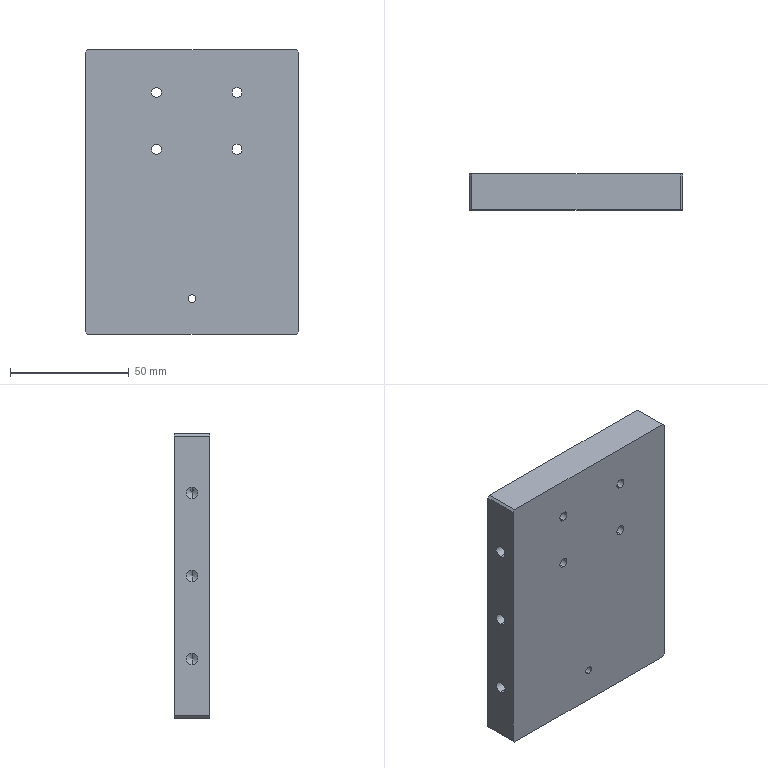Part | SolidWorks | features BaseBody 1 | 1 solid | 40 faces | box 90 x 15 x 120 mm | volume 159292 mm3 | cylinder 20 | cone 10 | plane 10 | commonest cylinder face diameters 5 x10 4.2 x8 3.3 x2
STEP:
#1=CARTESIAN_POINT('',(64.,15.,-39.9));
#2=VERTEX_POINT('',#1);
#3=CARTESIAN_POINT('',(64.,15.,-44.1));
#4=VERTEX_POINT('',#3);
#5=CARTESIAN_POINT('',(64.,15.,-42.));
#6=DIRECTION('',(0.,-1.,0.));
#7=DIRECTION('',(0.,0.,-1.));
#8=AXIS2_PLACEMENT_3D('',#5,#6,#7);
#9=CIRCLE('',#8,2.1);
#10=EDGE_CURVE('',#2,#4,#9,.T.);
#11=ORIENTED_EDGE('',*,*,#10,.F.);
#12=CARTESIAN_POINT('',(64.,0.,-39.9));
#13=VERTEX_POINT('',#12);
#14=CARTESIAN_POINT('',(64.,0.,-39.9));
#15=DIRECTION('',(0.,-1.,0.));
#16=VECTOR('',#15,1000.);
#17=LINE('',#14,#16);
#18=EDGE_CURVE('',#2,#13,#17,.T.);
#19=ORIENTED_EDGE('',*,*,#18,.T.);
#20=CARTESIAN_POINT('',(64.,0.,-44.1));
#21=VERTEX_POINT('',#20);
#22=CARTESIAN_POINT('',(64.,0.,-42.));
#23=DIRECTION('',(0.,1.,0.));
#24=DIRECTION('',(0.,0.,-1.));
#25=AXIS2_PLACEMENT_3D('',#22,#23,#24);
#26=CIRCLE('',#25,2.1);
#27=EDGE_CURVE('',#21,#13,#26,.T.);
#28=ORIENTED_EDGE('',*,*,#27,.F.);
#29=CARTESIAN_POINT('',(64.,0.,-44.1));
#30=DIRECTION('',(0.,-1.,0.));
#31=VECTOR('',#30,1000.);
#32=LINE('',#29,#31);
#33=EDGE_CURVE('',#4,#21,#32,.T.);
#34=ORIENTED_EDGE('',*,*,#33,.F.);
#35=EDGE_LOOP('',(#11,#19,#28,#34));
#36=FACE_OUTER_BOUND('',#35,.T.);
#37=CARTESIAN_POINT('',(64.,0.,-42.));
#38=DIRECTION('',(0.,-1.,0.));
#39=DIRECTION('',(0.,0.,-1.));
#40=AXIS2_PLACEMENT_3D('',#37,#38,#39);
#41=CYLINDRICAL_SURFACE('',#40,2.1);
#42=ADVANCED_FACE('',(#36),#41,.F.);
#43=CARTESIAN_POINT('',(64.,15.,-15.9));
#44=VERTEX_POINT('',#43);
#45=CARTESIAN_POINT('',(64.,15.,-20.1));
#46=VERTEX_POINT('',#45);
#47=CARTESIAN_POINT('',(64.,15.,-18.));
#48=DIRECTION('',(0.,-1.,0.));
#49=DIRECTION('',(0.,0.,-1.));
#50=AXIS2_PLACEMENT_3D('',#47,#48,#49);
#51=CIRCLE('',#50,2.1);
#52=EDGE_CURVE('',#44,#46,#51,.T.);
#53=ORIENTED_EDGE('',*,*,#52,.F.);
#54=CARTESIAN_POINT('',(64.,0.,-15.9));
#55=VERTEX_POINT('',#54);
#56=CARTESIAN_POINT('',(64.,0.,-15.9));
#57=DIRECTION('',(0.,-1.,0.));
#58=VECTOR('',#57,1000.);
#59=LINE('',#56,#58);
#60=EDGE_CURVE('',#44,#55,#59,.T.);
#61=ORIENTED_EDGE('',*,*,#60,.T.);
#62=CARTESIAN_POINT('',(64.,0.,-20.1));
#63=VERTEX_POINT('',#62);
#64=CARTESIAN_POINT('',(64.,0.,-18.));
#65=DIRECTION('',(0.,1.,0.));
#66=DIRECTION('',(0.,0.,-1.));
#67=AXIS2_PLACEMENT_3D('',#64,#65,#66);
#68=CIRCLE('',#67,2.1);
#69=EDGE_CURVE('',#63,#55,#68,.T.);
#70=ORIENTED_EDGE('',*,*,#69,.F.);
#71=CARTESIAN_POINT('',(64.,0.,-20.1));
#72=DIRECTION('',(0.,-1.,0.));
#73=VECTOR('',#72,1000.);
#74=LINE('',#71,#73);
#75=EDGE_CURVE('',#46,#63,#74,.T.);
#76=ORIENTED_EDGE('',*,*,#75,.F.);
#77=EDGE_LOOP('',(#53,#61,#70,#76));
#78=FACE_OUTER_BOUND('',#77,.T.);
#79=CARTESIAN_POINT('',(64.,0.,-18.));
#80=DIRECTION('',(0.,-1.,0.));
#81=DIRECTION('',(0.,0.,-1.));
#82=AXIS2_PLACEMENT_3D('',#79,#80,#81);
#83=CYLINDRICAL_SURFACE('',#82,2.1);
#84=ADVANCED_FACE('',(#78),#83,.F.);
#85=CARTESIAN_POINT('',(30.,15.,-15.9));
#86=VERTEX_POINT('',#85);
#87=CARTESIAN_POINT('',(30.,15.,-20.1));
#88=VERTEX_POINT('',#87);
#89=CARTESIAN_POINT('',(30.,15.,-18.));
#90=DIRECTION('',(0.,-1.,0.));
#91=DIRECTION('',(0.,0.,-1.));
#92=AXIS2_PLACEMENT_3D('',#89,#90,#91);
#93=CIRCLE('',#92,2.1);
#94=EDGE_CURVE('',#86,#88,#93,.T.);
#95=ORIENTED_EDGE('',*,*,#94,.F.);
#96=CARTESIAN_POINT('',(30.,0.,-15.9));
#97=VERTEX_POINT('',#96);
#98=CARTESIAN_POINT('',(30.,0.,-15.9));
#99=DIRECTION('',(0.,-1.,0.));
#100=VECTOR('',#99,1000.);
#101=LINE('',#98,#100);
#102=EDGE_CURVE('',#86,#97,#101,.T.);
#103=ORIENTED_EDGE('',*,*,#102,.T.);
#104=CARTESIAN_POINT('',(30.,0.,-20.1));
#105=VERTEX_POINT('',#104);
#106=CARTESIAN_POINT('',(30.,0.,-18.));
#107=DIRECTION('',(0.,1.,0.));
#108=DIRECTION('',(0.,0.,-1.));
#109=AXIS2_PLACEMENT_3D('',#106,#107,#108);
#110=CIRCLE('',#109,2.1);
#111=EDGE_CURVE('',#105,#97,#110,.T.);
#112=ORIENTED_EDGE('',*,*,#111,.F.);
#113=CARTESIAN_POINT('',(30.,0.,-20.1));
#114=DIRECTION('',(0.,-1.,0.));
#115=VECTOR('',#114,1000.);
#116=LINE('',#113,#115);
#117=EDGE_CURVE('',#88,#105,#116,.T.);
#118=ORIENTED_EDGE('',*,*,#117,.F.);
#119=EDGE_LOOP('',(#95,#103,#112,#118));
#120=FACE_OUTER_BOUND('',#119,.T.);
#121=CARTESIAN_POINT('',(30.,0.,-18.));
#122=DIRECTION('',(0.,-1.,0.));
#123=DIRECTION('',(0.,0.,-1.));
#124=AXIS2_PLACEMENT_3D('',#121,#122,#123);
#125=CYLINDRICAL_SURFACE('',#124,2.1);
#126=ADVANCED_FACE('',(#120),#125,.F.);
#127=CARTESIAN_POINT('',(30.,15.,-39.9));
#128=VERTEX_POINT('',#127);
#129=CARTESIAN_POINT('',(30.,15.,-44.1));
#130=VERTEX_POINT('',#129);
#131=CARTESIAN_POINT('',(30.,15.,-42.));
#132=DIRECTION('',(0.,-1.,0.));
#133=DIRECTION('',(0.,0.,-1.));
#134=AXIS2_PLACEMENT_3D('',#131,#132,#133);
#135=CIRCLE('',#134,2.1);
#136=EDGE_CURVE('',#128,#130,#135,.T.);
#137=ORIENTED_EDGE('',*,*,#136,.F.);
#138=CARTESIAN_POINT('',(30.,0.,-39.9));
#139=VERTEX_POINT('',#138);
#140=CARTESIAN_POINT('',(30.,0.,-39.9));
#141=DIRECTION('',(0.,-1.,0.));
#142=VECTOR('',#141,1000.);
#143=LINE('',#140,#142);
#144=EDGE_CURVE('',#128,#139,#143,.T.);
#145=ORIENTED_EDGE('',*,*,#144,.T.);
#146=CARTESIAN_POINT('',(30.,0.,-44.1));
#147=VERTEX_POINT('',#146);
#148=CARTESIAN_POINT('',(30.,0.,-42.));
#149=DIRECTION('',(0.,1.,0.));
#150=DIRECTION('',(0.,0.,-1.));
#151=AXIS2_PLACEMENT_3D('',#148,#149,#150);
#152=CIRCLE('',#151,2.1);
#153=EDGE_CURVE('',#147,#139,#152,.T.);
#154=ORIENTED_EDGE('',*,*,#153,.F.);
#155=CARTESIAN_POINT('',(30.,0.,-44.1));
#156=DIRECTION('',(0.,-1.,0.));
#157=VECTOR('',#156,1000.);
#158=LINE('',#155,#157);
#159=EDGE_CURVE('',#130,#147,#158,.T.);
#160=ORIENTED_EDGE('',*,*,#159,.F.);
#161=EDGE_LOOP('',(#137,#145,#154,#160));
#162=FACE_OUTER_BOUND('',#161,.T.);
#163=CARTESIAN_POINT('',(30.,0.,-42.));
#164=DIRECTION('',(0.,-1.,0.));
#165=DIRECTION('',(0.,0.,-1.));
#166=AXIS2_PLACEMENT_3D('',#163,#164,#165);
#167=CYLINDRICAL_SURFACE('',#166,2.1);
#168=ADVANCED_FACE('',(#162),#167,.F.);
#169=CARTESIAN_POINT('',(45.,0.,-106.65));
#170=VERTEX_POINT('',#169);
#171=CARTESIAN_POINT('',(45.,0.,-103.35));
#172=VERTEX_POINT('',#171);
#173=CARTESIAN_POINT('',(45.,0.,-105.));
#174=DIRECTION('',(0.,1.,0.));
#175=DIRECTION('',(0.,0.,1.));
#176=AXIS2_PLACEMENT_3D('',#173,#174,#175);
#177=CIRCLE('',#176,1.65);
#178=EDGE_CURVE('',#170,#172,#177,.T.);
#179=ORIENTED_EDGE('',*,*,#178,.F.);
#180=CARTESIAN_POINT('',(45.,15.,-106.65));
#181=VERTEX_POINT('',#180);
#182=CARTESIAN_POINT('',(45.,15.,-106.65));
#183=DIRECTION('',(0.,1.,0.));
#184=VECTOR('',#183,1000.);
#185=LINE('',#182,#184);
#186=EDGE_CURVE('',#170,#181,#185,.T.);
#187=ORIENTED_EDGE('',*,*,#186,.T.);
#188=CARTESIAN_POINT('',(45.,15.,-103.35));
#189=VERTEX_POINT('',#188);
#190=CARTESIAN_POINT('',(45.,15.,-105.));
#191=DIRECTION('',(0.,-1.,0.));
#192=DIRECTION('',(0.,0.,1.));
#193=AXIS2_PLACEMENT_3D('',#190,#191,#192);
#194=CIRCLE('',#193,1.65);
#195=EDGE_CURVE('',#189,#181,#194,.T.);
#196=ORIENTED_EDGE('',*,*,#195,.F.);
#197=CARTESIAN_POINT('',(45.,15.,-103.35));
#198=DIRECTION('',(0.,1.,0.));
#199=VECTOR('',#198,1000.);
#200=LINE('',#197,#199);
#201=EDGE_CURVE('',#172,#189,#200,.T.);
#202=ORIENTED_EDGE('',*,*,#201,.F.);
#203=EDGE_LOOP('',(#179,#187,#196,#202));
#204=FACE_OUTER_BOUND('',#203,.T.);
#205=CARTESIAN_POINT('',(45.,15.,-105.));
#206=DIRECTION('',(0.,1.,0.));
#207=DIRECTION('',(0.,0.,1.));
#208=AXIS2_PLACEMENT_3D('',#205,#206,#207);
#209=CYLINDRICAL_SURFACE('',#208,1.65);
#210=ADVANCED_FACE('',(#204),#209,.F.);
#211=CARTESIAN_POINT('',(77.5,7.5,-103.));
#212=VERTEX_POINT('',#211);
#213=CARTESIAN_POINT('',(75.,5.,-103.));
#214=VERTEX_POINT('',#213);
#215=CARTESIAN_POINT('',(75.,7.5,-103.));
#216=DIRECTION('',(0.,0.,-1.));
#217=DIRECTION('',(-1.,0.,0.));
#218=AXIS2_PLACEMENT_3D('',#215,#216,#217);
#219=CIRCLE('',#218,2.5);
#220=EDGE_CURVE('',#212,#214,#219,.T.);
#221=ORIENTED_EDGE('',*,*,#220,.F.);
#222=CARTESIAN_POINT('',(77.5,7.5,-120.));
#223=VERTEX_POINT('',#222);
#224=CARTESIAN_POINT('',(77.5,7.5,-120.));
#225=DIRECTION('',(0.,0.,-1.));
#226=VECTOR('',#225,1000.);
#227=LINE('',#224,#226);
#228=EDGE_CURVE('',#212,#223,#227,.T.);
#229=ORIENTED_EDGE('',*,*,#228,.T.);
#230=CARTESIAN_POINT('',(72.5,7.5,-120.));
#231=VERTEX_POINT('',#230);
#232=CARTESIAN_POINT('',(75.,7.5,-120.));
#233=DIRECTION('',(0.,0.,-1.));
#234=DIRECTION('',(-1.,0.,0.));
#235=AXIS2_PLACEMENT_3D('',#232,#233,#234);
#236=CIRCLE('',#235,2.5);
#237=EDGE_CURVE('',#223,#231,#236,.T.);
#238=ORIENTED_EDGE('',*,*,#237,.T.);
#239=CARTESIAN_POINT('',(72.5,7.5,-103.));
#240=VERTEX_POINT('',#239);
#241=CARTESIAN_POINT('',(72.5,7.5,-120.));
#242=DIRECTION('',(0.,0.,-1.));
#243=VECTOR('',#242,1000.);
#244=LINE('',#241,#243);
#245=EDGE_CURVE('',#240,#231,#244,.T.);
#246=ORIENTED_EDGE('',*,*,#245,.F.);
#247=CARTESIAN_POINT('',(75.,7.5,-103.));
#248=DIRECTION('',(0.,0.,-1.));
#249=DIRECTION('',(-1.,0.,0.));
#250=AXIS2_PLACEMENT_3D('',#247,#248,#249);
#251=CIRCLE('',#250,2.5);
#252=EDGE_CURVE('',#214,#240,#251,.T.);
#253=ORIENTED_EDGE('',*,*,#252,.F.);
#254=EDGE_LOOP('',(#221,#229,#238,#246,#253));
#255=FACE_OUTER_BOUND('',#254,.T.);
#256=CARTESIAN_POINT('',(75.,7.5,-120.));
#257=DIRECTION('',(0.,0.,-1.));
#258=DIRECTION('',(-1.,0.,0.));
#259=AXIS2_PLACEMENT_3D('',#256,#257,#258);
#260=CYLINDRICAL_SURFACE('',#259,2.5);
#261=ADVANCED_FACE('',(#255),#260,.F.);
#262=CARTESIAN_POINT('',(17.5,7.5,-103.));
#263=VERTEX_POINT('',#262);
#264=CARTESIAN_POINT('',(12.5,7.5,-103.));
#265=VERTEX_POINT('',#264);
#266=CARTESIAN_POINT('',(15.,7.5,-103.));
#267=DIRECTION('',(0.,0.,-1.));
#268=DIRECTION('',(-1.,0.,0.));
#269=AXIS2_PLACEMENT_3D('',#266,#267,#268);
#270=CIRCLE('',#269,2.5);
#271=EDGE_CURVE('',#263,#265,#270,.T.);
#272=ORIENTED_EDGE('',*,*,#271,.F.);
#273=CARTESIAN_POINT('',(17.5,7.5,-120.));
#274=VERTEX_POINT('',#273);
#275=CARTESIAN_POINT('',(17.5,7.5,-120.));
#276=DIRECTION('',(0.,0.,-1.));
#277=VECTOR('',#276,1000.);
#278=LINE('',#275,#277);
#279=EDGE_CURVE('',#263,#274,#278,.T.);
#280=ORIENTED_EDGE('',*,*,#279,.T.);
#281=CARTESIAN_POINT('',(12.5,7.5,-120.));
#282=VERTEX_POINT('',#281);
#283=CARTESIAN_POINT('',(15.,7.5,-120.));
#284=DIRECTION('',(0.,0.,-1.));
#285=DIRECTION('',(-1.,0.,0.));
#286=AXIS2_PLACEMENT_3D('',#283,#284,#285);
#287=CIRCLE('',#286,2.5);
#288=EDGE_CURVE('',#274,#282,#287,.T.);
#289=ORIENTED_EDGE('',*,*,#288,.T.);
#290=CARTESIAN_POINT('',(12.5,7.5,-120.));
#291=DIRECTION('',(0.,0.,-1.));
#292=VECTOR('',#291,1000.);
#293=LINE('',#290,#292);
#294=EDGE_CURVE('',#265,#282,#293,.T.);
#295=ORIENTED_EDGE('',*,*,#294,.F.);
#296=EDGE_LOOP('',(#272,#280,#289,#295));
#297=FACE_OUTER_BOUND('',#296,.T.);
#298=CARTESIAN_POINT('',(15.,7.5,-120.));
#299=DIRECTION('',(0.,0.,-1.));
#300=DIRECTION('',(-1.,0.,0.));
#301=AXIS2_PLACEMENT_3D('',#298,#299,#300);
#302=CYLINDRICAL_SURFACE('',#301,2.5);
#303=ADVANCED_FACE('',(#297),#302,.F.);
#304=CARTESIAN_POINT('',(17.,7.5,-27.5));
#305=VERTEX_POINT('',#304);
#306=CARTESIAN_POINT('',(17.,7.5,-22.5));
#307=VERTEX_POINT('',#306);
#308=CARTESIAN_POINT('',(17.,7.5,-25.));
#309=DIRECTION('',(-1.,0.,0.));
#310=DIRECTION('',(0.,0.,1.));
#311=AXIS2_PLACEMENT_3D('',#308,#309,#310);
#312=CIRCLE('',#311,2.5);
#313=EDGE_CURVE('',#305,#307,#312,.T.);
#314=ORIENTED_EDGE('',*,*,#313,.F.);
#315=CARTESIAN_POINT('',(0.,7.5,-27.5));
#316=VERTEX_POINT('',#315);
#317=CARTESIAN_POINT('',(0.,7.5,-27.5));
#318=DIRECTION('',(-1.,0.,0.));
#319=VECTOR('',#318,1000.);
#320=LINE('',#317,#319);
#321=EDGE_CURVE('',#305,#316,#320,.T.);
#322=ORIENTED_EDGE('',*,*,#321,.T.);
#323=CARTESIAN_POINT('',(0.,7.5,-22.5));
#324=VERTEX_POINT('',#323);
#325=CARTESIAN_POINT('',(0.,7.5,-25.));
#326=DIRECTION('',(-1.,0.,0.));
#327=DIRECTION('',(0.,0.,1.));
#328=AXIS2_PLACEMENT_3D('',#325,#326,#327);
#329=CIRCLE('',#328,2.5);
#330=EDGE_CURVE('',#316,#324,#329,.T.);
#331=ORIENTED_EDGE('',*,*,#330,.T.);
#332=CARTESIAN_POINT('',(0.,7.5,-22.5));
#333=DIRECTION('',(-1.,0.,0.));
#334=VECTOR('',#333,1000.);
#335=LINE('',#332,#334);
#336=EDGE_CURVE('',#307,#324,#335,.T.);
#337=ORIENTED_EDGE('',*,*,#336,.F.);
#338=EDGE_LOOP('',(#314,#322,#331,#337));
#339=FACE_OUTER_BOUND('',#338,.T.);
#340=CARTESIAN_POINT('',(0.,7.5,-25.));
#341=DIRECTION('',(-1.,0.,0.));
#342=DIRECTION('',(0.,0.,1.));
#343=AXIS2_PLACEMENT_3D('',#340,#341,#342);
#344=CYLINDRICAL_SURFACE('',#343,2.5);
#345=ADVANCED_FACE('',(#339),#344,.F.);
#346=CARTESIAN_POINT('',(17.,7.5,-97.5));
#347=VERTEX_POINT('',#346);
#348=CARTESIAN_POINT('',(17.,7.5,-92.5));
#349=VERTEX_POINT('',#348);
#350=CARTESIAN_POINT('',(17.,7.5,-95.));
#351=DIRECTION('',(-1.,0.,0.));
#352=DIRECTION('',(0.,0.,1.));
#353=AXIS2_PLACEMENT_3D('',#350,#351,#352);
#354=CIRCLE('',#353,2.5);
#355=EDGE_CURVE('',#347,#349,#354,.T.);
#356=ORIENTED_EDGE('',*,*,#355,.F.);
#357=CARTESIAN_POINT('',(0.,7.5,-97.5));
#358=VERTEX_POINT('',#357);
#359=CARTESIAN_POINT('',(0.,7.5,-97.5));
#360=DIRECTION('',(-1.,0.,0.));
#361=VECTOR('',#360,1000.);
#362=LINE('',#359,#361);
#363=EDGE_CURVE('',#347,#358,#362,.T.);
#364=ORIENTED_EDGE('',*,*,#363,.T.);
#365=CARTESIAN_POINT('',(0.,7.5,-92.5));
#366=VERTEX_POINT('',#365);
#367=CARTESIAN_POINT('',(0.,7.5,-95.));
#368=DIRECTION('',(-1.,0.,0.));
#369=DIRECTION('',(0.,0.,1.));
#370=AXIS2_PLACEMENT_3D('',#367,#368,#369);
#371=CIRCLE('',#370,2.5);
#372=EDGE_CURVE('',#358,#366,#371,.T.);
#373=ORIENTED_EDGE('',*,*,#372,.T.);
#374=CARTESIAN_POINT('',(0.,7.5,-92.5));
#375=DIRECTION('',(-1.,0.,0.));
#376=VECTOR('',#375,1000.);
#377=LINE('',#374,#376);
#378=EDGE_CURVE('',#349,#366,#377,.T.);
#379=ORIENTED_EDGE('',*,*,#378,.F.);
#380=EDGE_LOOP('',(#356,#364,#373,#379));
#381=FACE_OUTER_BOUND('',#380,.T.);
#382=CARTESIAN_POINT('',(0.,7.5,-95.));
#383=DIRECTION('',(-1.,0.,0.));
#384=DIRECTION('',(0.,0.,1.));
#385=AXIS2_PLACEMENT_3D('',#382,#383,#384);
#386=CYLINDRICAL_SURFACE('',#385,2.5);
#387=ADVANCED_FACE('',(#381),#386,.F.);
#388=CARTESIAN_POINT('',(17.,7.5,-62.5));
#389=VERTEX_POINT('',#388);
#390=CARTESIAN_POINT('',(17.,7.5,-57.5));
#391=VERTEX_POINT('',#390);
#392=CARTESIAN_POINT('',(17.,7.5,-60.));
#393=DIRECTION('',(-1.,0.,0.));
#394=DIRECTION('',(0.,0.,1.));
#395=AXIS2_PLACEMENT_3D('',#392,#393,#394);
#396=CIRCLE('',#395,2.5);
#397=EDGE_CURVE('',#389,#391,#396,.T.);
#398=ORIENTED_EDGE('',*,*,#397,.F.);
#399=CARTESIAN_POINT('',(0.,7.5,-62.5));
#400=VERTEX_POINT('',#399);
#401=CARTESIAN_POINT('',(0.,7.5,-62.5));
#402=DIRECTION('',(-1.,0.,0.));
#403=VECTOR('',#402,1000.);
#404=LINE('',#401,#403);
#405=EDGE_CURVE('',#389,#400,#404,.T.);
#406=ORIENTED_EDGE('',*,*,#405,.T.);
#407=CARTESIAN_POINT('',(0.,7.5,-57.5));
#408=VERTEX_POINT('',#407);
#409=CARTESIAN_POINT('',(0.,7.5,-60.));
#410=DIRECTION('',(-1.,0.,0.));
#411=DIRECTION('',(0.,0.,1.));
#412=AXIS2_PLACEMENT_3D('',#409,#410,#411);
#413=CIRCLE('',#412,2.5);
#414=EDGE_CURVE('',#400,#408,#413,.T.);
#415=ORIENTED_EDGE('',*,*,#414,.T.);
#416=CARTESIAN_POINT('',(0.,7.5,-57.5));
#417=DIRECTION('',(-1.,0.,0.));
#418=VECTOR('',#417,1000.);
#419=LINE('',#416,#418);
#420=EDGE_CURVE('',#391,#408,#419,.T.);
#421=ORIENTED_EDGE('',*,*,#420,.F.);
#422=EDGE_LOOP('',(#398,#406,#415,#421));
#423=FACE_OUTER_BOUND('',#422,.T.);
#424=CARTESIAN_POINT('',(0.,7.5,-60.));
#425=DIRECTION('',(-1.,0.,0.));
#426=DIRECTION('',(0.,0.,1.));
#427=AXIS2_PLACEMENT_3D('',#424,#425,#426);
#428=CYLINDRICAL_SURFACE('',#427,2.5);
#429=ADVANCED_FACE('',(#423),#428,.F.);
#430=CARTESIAN_POINT('',(75.,7.5,-101.498));
#431=VERTEX_POINT('',#430);
#432=CARTESIAN_POINT('',(75.,10.,-103.));
#433=VERTEX_POINT('',#432);
#434=CARTESIAN_POINT('',(75.,10.,-103.));
#435=DIRECTION('',(0.,0.8572,-0.515));
#436=VECTOR('',#435,1000.);
#437=LINE('',#434,#436);
#438=EDGE_CURVE('',#431,#433,#437,.T.);
#439=ORIENTED_EDGE('',*,*,#438,.F.);
#440=CARTESIAN_POINT('',(75.,5.,-103.));
#441=DIRECTION('',(0.,-0.8572,-0.515));
#442=VECTOR('',#441,1000.);
#443=LINE('',#440,#442);
#444=EDGE_CURVE('',#431,#214,#443,.T.);
#445=ORIENTED_EDGE('',*,*,#444,.T.);
#446=ORIENTED_EDGE('',*,*,#252,.T.);
#447=CARTESIAN_POINT('',(75.,7.5,-103.));
#448=DIRECTION('',(0.,0.,-1.));
#449=DIRECTION('',(-1.,0.,0.));
#450=AXIS2_PLACEMENT_3D('',#447,#448,#449);
#451=CIRCLE('',#450,2.5);
#452=EDGE_CURVE('',#240,#433,#451,.T.);
#453=ORIENTED_EDGE('',*,*,#452,.T.);
#454=EDGE_LOOP('',(#439,#445,#446,#453));
#455=FACE_OUTER_BOUND('',#454,.T.);
#456=CARTESIAN_POINT('',(75.,7.5,-103.));
#457=DIRECTION('',(0.,0.,-1.));
#458=DIRECTION('',(0.,1.,0.));
#459=AXIS2_PLACEMENT_3D('',#456,#457,#458);
#460=CONICAL_SURFACE('',#459,2.5,1.03);
#461=ADVANCED_FACE('',(#455),#460,.F.);
#462=CARTESIAN_POINT('',(15.,7.5,-101.498));
#463=VERTEX_POINT('',#462);
#464=CARTESIAN_POINT('',(12.5,7.5,-103.));
#465=DIRECTION('',(-0.8572,0.,-0.515));
#466=VECTOR('',#465,1000.);
#467=LINE('',#464,#466);
#468=EDGE_CURVE('',#463,#265,#467,.T.);
#469=ORIENTED_EDGE('',*,*,#468,.F.);
#470=CARTESIAN_POINT('',(17.5,7.5,-103.));
#471=DIRECTION('',(0.8572,0.,-0.515));
#472=VECTOR('',#471,1000.);
#473=LINE('',#470,#472);
#474=EDGE_CURVE('',#463,#263,#473,.T.);
#475=ORIENTED_EDGE('',*,*,#474,.T.);
#476=ORIENTED_EDGE('',*,*,#271,.T.);
#477=EDGE_LOOP('',(#469,#475,#476));
#478=FACE_OUTER_BOUND('',#477,.T.);
#479=CARTESIAN_POINT('',(15.,7.5,-103.));
#480=DIRECTION('',(0.,0.,-1.));
#481=DIRECTION('',(-1.,0.,0.));
#482=AXIS2_PLACEMENT_3D('',#479,#480,#481);
#483=CONICAL_SURFACE('',#482,2.5,1.03);
#484=ADVANCED_FACE('',(#478),#483,.F.);
#485=CARTESIAN_POINT('',(18.502,7.5,-25.));
#486=VERTEX_POINT('',#485);
#487=CARTESIAN_POINT('',(17.,7.5,-22.5));
#488=DIRECTION('',(-0.515,0.,0.8572));
#489=VECTOR('',#488,1000.);
#490=LINE('',#487,#489);
#491=EDGE_CURVE('',#486,#307,#490,.T.);
#492=ORIENTED_EDGE('',*,*,#491,.F.);
#493=CARTESIAN_POINT('',(17.,7.5,-27.5));
#494=DIRECTION('',(-0.515,0.,-0.8572));
#495=VECTOR('',#494,1000.);
#496=LINE('',#493,#495);
#497=EDGE_CURVE('',#486,#305,#496,.T.);
#498=ORIENTED_EDGE('',*,*,#497,.T.);
#499=ORIENTED_EDGE('',*,*,#313,.T.);
#500=EDGE_LOOP('',(#492,#498,#499));
#501=FACE_OUTER_BOUND('',#500,.T.);
#502=CARTESIAN_POINT('',(17.,7.5,-25.));
#503=DIRECTION('',(-1.,0.,0.));
#504=DIRECTION('',(0.,0.,1.));
#505=AXIS2_PLACEMENT_3D('',#502,#503,#504);
#506=CONICAL_SURFACE('',#505,2.5,1.03);
#507=ADVANCED_FACE('',(#501),#506,.F.);
#508=CARTESIAN_POINT('',(18.502,7.5,-95.));
#509=VERTEX_POINT('',#508);
#510=CARTESIAN_POINT('',(17.,7.5,-92.5));
#511=DIRECTION('',(-0.515,0.,0.8572));
#512=VECTOR('',#511,1000.);
#513=LINE('',#510,#512);
#514=EDGE_CURVE('',#509,#349,#513,.T.);
#515=ORIENTED_EDGE('',*,*,#514,.F.);
#516=CARTESIAN_POINT('',(17.,7.5,-97.5));
#517=DIRECTION('',(-0.515,0.,-0.8572));
#518=VECTOR('',#517,1000.);
#519=LINE('',#516,#518);
#520=EDGE_CURVE('',#509,#347,#519,.T.);
#521=ORIENTED_EDGE('',*,*,#520,.T.);
#522=ORIENTED_EDGE('',*,*,#355,.T.);
#523=EDGE_LOOP('',(#515,#521,#522));
#524=FACE_OUTER_BOUND('',#523,.T.);
#525=CARTESIAN_POINT('',(17.,7.5,-95.));
#526=DIRECTION('',(-1.,0.,0.));
#527=DIRECTION('',(0.,0.,1.));
#528=AXIS2_PLACEMENT_3D('',#525,#526,#527);
#529=CONICAL_SURFACE('',#528,2.5,1.03);
#530=ADVANCED_FACE('',(#524),#529,.F.);
#531=CARTESIAN_POINT('',(18.502,7.5,-60.));
#532=VERTEX_POINT('',#531);
#533=CARTESIAN_POINT('',(17.,7.5,-57.5));
#534=DIRECTION('',(-0.515,0.,0.8572));
#535=VECTOR('',#534,1000.);
#536=LINE('',#533,#535);
#537=EDGE_CURVE('',#532,#391,#536,.T.);
#538=ORIENTED_EDGE('',*,*,#537,.F.);
#539=CARTESIAN_POINT('',(17.,7.5,-62.5));
#540=DIRECTION('',(-0.515,0.,-0.8572));
#541=VECTOR('',#540,1000.);
#542=LINE('',#539,#541);
#543=EDGE_CURVE('',#532,#389,#542,.T.);
#544=ORIENTED_EDGE('',*,*,#543,.T.);
#545=ORIENTED_EDGE('',*,*,#397,.T.);
#546=EDGE_LOOP('',(#538,#544,#545));
#547=FACE_OUTER_BOUND('',#546,.T.);
#548=CARTESIAN_POINT('',(17.,7.5,-60.));
#549=DIRECTION('',(-1.,0.,0.));
#550=DIRECTION('',(0.,0.,1.));
#551=AXIS2_PLACEMENT_3D('',#548,#549,#550);
#552=CONICAL_SURFACE('',#551,2.5,1.03);
#553=ADVANCED_FACE('',(#547),#552,.F.);
#554=CARTESIAN_POINT('',(90.,0.,-119.));
#555=VERTEX_POINT('',#554);
#556=CARTESIAN_POINT('',(90.,0.,-1.));
#557=VERTEX_POINT('',#556);
#558=CARTESIAN_POINT('',(90.,0.,0.));
#559=DIRECTION('',(0.,0.,1.));
#560=VECTOR('',#559,1000.);
#561=LINE('',#558,#560);
#562=EDGE_CURVE('',#555,#557,#561,.T.);
#563=ORIENTED_EDGE('',*,*,#562,.T.);
#564=CARTESIAN_POINT('',(89.,0.,0.));
#565=VERTEX_POINT('',#564);
#566=CARTESIAN_POINT('',(90.,0.,-1.));
#567=DIRECTION('',(-0.7071,0.,0.7071));
#568=VECTOR('',#567,1000.);
#569=LINE('',#566,#568);
#570=EDGE_CURVE('',#557,#565,#569,.T.);
#571=ORIENTED_EDGE('',*,*,#570,.T.);
#572=CARTESIAN_POINT('',(1.,0.,0.));
#573=VERTEX_POINT('',#572);
#574=CARTESIAN_POINT('',(0.,0.,0.));
#575=DIRECTION('',(-1.,0.,0.));
#576=VECTOR('',#575,1000.);
#577=LINE('',#574,#576);
#578=EDGE_CURVE('',#565,#573,#577,.T.);
#579=ORIENTED_EDGE('',*,*,#578,.T.);
#580=CARTESIAN_POINT('',(0.,0.,-1.));
#581=VERTEX_POINT('',#580);
#582=CARTESIAN_POINT('',(1.,0.,0.));
#583=DIRECTION('',(-0.7071,0.,-0.7071));
#584=VECTOR('',#583,1000.);
#585=LINE('',#582,#584);
#586=EDGE_CURVE('',#573,#581,#585,.T.);
#587=ORIENTED_EDGE('',*,*,#586,.T.);
#588=CARTESIAN_POINT('',(0.,0.,-119.));
#589=VERTEX_POINT('',#588);
#590=CARTESIAN_POINT('',(0.,0.,0.));
#591=DIRECTION('',(0.,0.,-1.));
#592=VECTOR('',#591,1000.);
#593=LINE('',#590,#592);
#594=EDGE_CURVE('',#581,#589,#593,.T.);
#595=ORIENTED_EDGE('',*,*,#594,.T.);
#596=CARTESIAN_POINT('',(1.,0.,-120.));
#597=VERTEX_POINT('',#596);
#598=CARTESIAN_POINT('',(0.,0.,-119.));
#599=DIRECTION('',(0.7071,0.,-0.7071));
#600=VECTOR('',#599,1000.);
#601=LINE('',#598,#600);
#602=EDGE_CURVE('',#589,#597,#601,.T.);
#603=ORIENTED_EDGE('',*,*,#602,.T.);
#604=CARTESIAN_POINT('',(89.,0.,-120.));
#605=VERTEX_POINT('',#604);
#606=CARTESIAN_POINT('',(0.,0.,-120.));
#607=DIRECTION('',(1.,0.,0.));
#608=VECTOR('',#607,1000.);
#609=LINE('',#606,#608);
#610=EDGE_CURVE('',#597,#605,#609,.T.);
#611=ORIENTED_EDGE('',*,*,#610,.T.);
#612=CARTESIAN_POINT('',(89.,0.,-120.));
#613=DIRECTION('',(0.7071,0.,0.7071));
#614=VECTOR('',#613,1000.);
#615=LINE('',#612,#614);
#616=EDGE_CURVE('',#605,#555,#615,.T.);
#617=ORIENTED_EDGE('',*,*,#616,.T.);
#618=EDGE_LOOP('',(#563,#571,#579,#587,#595,#603,#611,#617));
#619=FACE_OUTER_BOUND('',#618,.T.);
#620=ORIENTED_EDGE('',*,*,#27,.T.);
#621=CARTESIAN_POINT('',(64.,0.,-42.));
#622=DIRECTION('',(0.,1.,0.));
#623=DIRECTION('',(0.,0.,-1.));
#624=AXIS2_PLACEMENT_3D('',#621,#622,#623);
#625=CIRCLE('',#624,2.1);
#626=EDGE_CURVE('',#13,#21,#625,.T.);
#627=ORIENTED_EDGE('',*,*,#626,.T.);
#628=EDGE_LOOP('',(#620,#627));
#629=FACE_BOUND('',#628,.T.);
#630=ORIENTED_EDGE('',*,*,#69,.T.);
#631=CARTESIAN_POINT('',(64.,0.,-18.));
#632=DIRECTION('',(0.,1.,0.));
#633=DIRECTION('',(0.,0.,-1.));
#634=AXIS2_PLACEMENT_3D('',#631,#632,#633);
#635=CIRCLE('',#634,2.1);
#636=EDGE_CURVE('',#55,#63,#635,.T.);
#637=ORIENTED_EDGE('',*,*,#636,.T.);
#638=EDGE_LOOP('',(#630,#637));
#639=FACE_BOUND('',#638,.T.);
#640=ORIENTED_EDGE('',*,*,#111,.T.);
#641=CARTESIAN_POINT('',(30.,0.,-18.));
#642=DIRECTION('',(0.,1.,0.));
#643=DIRECTION('',(0.,0.,-1.));
#644=AXIS2_PLACEMENT_3D('',#641,#642,#643);
#645=CIRCLE('',#644,2.1);
#646=EDGE_CURVE('',#97,#105,#645,.T.);
#647=ORIENTED_EDGE('',*,*,#646,.T.);
#648=EDGE_LOOP('',(#640,#647));
#649=FACE_BOUND('',#648,.T.);
#650=ORIENTED_EDGE('',*,*,#153,.T.);
#651=CARTESIAN_POINT('',(30.,0.,-42.));
#652=DIRECTION('',(0.,1.,0.));
#653=DIRECTION('',(0.,0.,-1.));
#654=AXIS2_PLACEMENT_3D('',#651,#652,#653);
#655=CIRCLE('',#654,2.1);
#656=EDGE_CURVE('',#139,#147,#655,.T.);
#657=ORIENTED_EDGE('',*,*,#656,.T.);
#658=EDGE_LOOP('',(#650,#657));
#659=FACE_BOUND('',#658,.T.);
#660=CARTESIAN_POINT('',(45.,0.,-105.));
#661=DIRECTION('',(0.,1.,0.));
#662=DIRECTION('',(0.,0.,1.));
#663=AXIS2_PLACEMENT_3D('',#660,#661,#662);
#664=CIRCLE('',#663,1.65);
#665=EDGE_CURVE('',#172,#170,#664,.T.);
#666=ORIENTED_EDGE('',*,*,#665,.T.);
#667=ORIENTED_EDGE('',*,*,#178,.T.);
#668=EDGE_LOOP('',(#666,#667));
#669=FACE_BOUND('',#668,.T.);
#670=CARTESIAN_POINT('',(0.,0.,0.));
#671=DIRECTION('',(0.,-1.,0.));
#672=DIRECTION('',(0.,0.,-1.));
#673=AXIS2_PLACEMENT_3D('',#670,#671,#672);
#674=PLANE('',#673);
#675=ADVANCED_FACE('',(#619,#629,#639,#649,#659,#669),#674,.T.);
#676=CARTESIAN_POINT('',(90.,15.,-119.));
#677=VERTEX_POINT('',#676);
#678=CARTESIAN_POINT('',(90.,15.,-119.));
#679=DIRECTION('',(0.,-1.,0.));
#680=VECTOR('',#679,1000.);
#681=LINE('',#678,#680);
#682=EDGE_CURVE('',#677,#555,#681,.T.);
#683=ORIENTED_EDGE('',*,*,#682,.F.);
#684=CARTESIAN_POINT('',(90.,15.,-1.));
#685=VERTEX_POINT('',#684);
#686=CARTESIAN_POINT('',(90.,15.,0.));
#687=DIRECTION('',(0.,0.,-1.));
#688=VECTOR('',#687,1000.);
#689=LINE('',#686,#688);
#690=EDGE_CURVE('',#685,#677,#689,.T.);
#691=ORIENTED_EDGE('',*,*,#690,.F.);
#692=CARTESIAN_POINT('',(90.,15.,-1.));
#693=DIRECTION('',(0.,1.,0.));
#694=VECTOR('',#693,1000.);
#695=LINE('',#692,#694);
#696=EDGE_CURVE('',#557,#685,#695,.T.);
#697=ORIENTED_EDGE('',*,*,#696,.F.);
#698=ORIENTED_EDGE('',*,*,#562,.F.);
#699=EDGE_LOOP('',(#683,#691,#697,#698));
#700=FACE_OUTER_BOUND('',#699,.T.);
#701=CARTESIAN_POINT('',(90.,15.,0.));
#702=DIRECTION('',(-1.,0.,0.));
#703=DIRECTION('',(0.,0.,1.));
#704=AXIS2_PLACEMENT_3D('',#701,#702,#703);
#705=PLANE('',#704);
#706=ADVANCED_FACE('',(#700),#705,.F.);
#707=CARTESIAN_POINT('',(1.,15.,-120.));
#708=VERTEX_POINT('',#707);
#709=CARTESIAN_POINT('',(1.,15.,-120.));
#710=DIRECTION('',(0.,-1.,0.));
#711=VECTOR('',#710,1000.);
#712=LINE('',#709,#711);
#713=EDGE_CURVE('',#708,#597,#712,.T.);
#714=ORIENTED_EDGE('',*,*,#713,.F.);
#715=CARTESIAN_POINT('',(89.,15.,-120.));
#716=VERTEX_POINT('',#715);
#717=CARTESIAN_POINT('',(0.,15.,-120.));
#718=DIRECTION('',(-1.,0.,0.));
#719=VECTOR('',#718,1000.);
#720=LINE('',#717,#719);
#721=EDGE_CURVE('',#716,#708,#720,.T.);
#722=ORIENTED_EDGE('',*,*,#721,.F.);
#723=CARTESIAN_POINT('',(89.,15.,-120.));
#724=DIRECTION('',(0.,1.,0.));
#725=VECTOR('',#724,1000.);
#726=LINE('',#723,#725);
#727=EDGE_CURVE('',#605,#716,#726,.T.);
#728=ORIENTED_EDGE('',*,*,#727,.F.);
#729=ORIENTED_EDGE('',*,*,#610,.F.);
#730=EDGE_LOOP('',(#714,#722,#728,#729));
#731=FACE_OUTER_BOUND('',#730,.T.);
#732=CARTESIAN_POINT('',(75.,7.5,-120.));
#733=DIRECTION('',(0.,0.,-1.));
#734=DIRECTION('',(-1.,0.,0.));
#735=AXIS2_PLACEMENT_3D('',#732,#733,#734);
#736=CIRCLE('',#735,2.5);
#737=EDGE_CURVE('',#231,#223,#736,.T.);
#738=ORIENTED_EDGE('',*,*,#737,.F.);
#739=ORIENTED_EDGE('',*,*,#237,.F.);
#740=EDGE_LOOP('',(#738,#739));
#741=FACE_BOUND('',#740,.T.);
#742=CARTESIAN_POINT('',(15.,7.5,-120.));
#743=DIRECTION('',(0.,0.,-1.));
#744=DIRECTION('',(-1.,0.,0.));
#745=AXIS2_PLACEMENT_3D('',#742,#743,#744);
#746=CIRCLE('',#745,2.5);
#747=EDGE_CURVE('',#282,#274,#746,.T.);
#748=ORIENTED_EDGE('',*,*,#747,.F.);
#749=ORIENTED_EDGE('',*,*,#288,.F.);
#750=EDGE_LOOP('',(#748,#749));
#751=FACE_BOUND('',#750,.T.);
#752=CARTESIAN_POINT('',(0.,15.,-120.));
#753=DIRECTION('',(0.,0.,1.));
#754=DIRECTION('',(1.,0.,0.));
#755=AXIS2_PLACEMENT_3D('',#752,#753,#754);
#756=PLANE('',#755);
#757=ADVANCED_FACE('',(#731,#741,#751),#756,.F.);
#758=CARTESIAN_POINT('',(0.,15.,-1.));
#759=VERTEX_POINT('',#758);
#760=CARTESIAN_POINT('',(0.,15.,-1.));
#761=DIRECTION('',(0.,-1.,0.));
#762=VECTOR('',#761,1000.);
#763=LINE('',#760,#762);
#764=EDGE_CURVE('',#759,#581,#763,.T.);
#765=ORIENTED_EDGE('',*,*,#764,.F.);
#766=CARTESIAN_POINT('',(0.,15.,-119.));
#767=VERTEX_POINT('',#766);
#768=CARTESIAN_POINT('',(0.,15.,0.));
#769=DIRECTION('',(0.,0.,1.));
#770=VECTOR('',#769,1000.);
#771=LINE('',#768,#770);
#772=EDGE_CURVE('',#767,#759,#771,.T.);
#773=ORIENTED_EDGE('',*,*,#772,.F.);
#774=CARTESIAN_POINT('',(0.,15.,-119.));
#775=DIRECTION('',(0.,1.,0.));
#776=VECTOR('',#775,1000.);
#777=LINE('',#774,#776);
#778=EDGE_CURVE('',#589,#767,#777,.T.);
#779=ORIENTED_EDGE('',*,*,#778,.F.);
#780=ORIENTED_EDGE('',*,*,#594,.F.);
#781=EDGE_LOOP('',(#765,#773,#779,#780));
#782=FACE_OUTER_BOUND('',#781,.T.);
#783=CARTESIAN_POINT('',(0.,7.5,-25.));
#784=DIRECTION('',(-1.,0.,0.));
#785=DIRECTION('',(0.,0.,1.));
#786=AXIS2_PLACEMENT_3D('',#783,#784,#785);
#787=CIRCLE('',#786,2.5);
#788=EDGE_CURVE('',#324,#316,#787,.T.);
#789=ORIENTED_EDGE('',*,*,#788,.F.);
#790=ORIENTED_EDGE('',*,*,#330,.F.);
#791=EDGE_LOOP('',(#789,#790));
#792=FACE_BOUND('',#791,.T.);
#793=CARTESIAN_POINT('',(0.,7.5,-95.));
#794=DIRECTION('',(-1.,0.,0.));
#795=DIRECTION('',(0.,0.,1.));
#796=AXIS2_PLACEMENT_3D('',#793,#794,#795);
#797=CIRCLE('',#796,2.5);
#798=EDGE_CURVE('',#366,#358,#797,.T.);
#799=ORIENTED_EDGE('',*,*,#798,.F.);
#800=ORIENTED_EDGE('',*,*,#372,.F.);
#801=EDGE_LOOP('',(#799,#800));
#802=FACE_BOUND('',#801,.T.);
#803=CARTESIAN_POINT('',(0.,7.5,-60.));
#804=DIRECTION('',(-1.,0.,0.));
#805=DIRECTION('',(0.,0.,1.));
#806=AXIS2_PLACEMENT_3D('',#803,#804,#805);
#807=CIRCLE('',#806,2.5);
#808=EDGE_CURVE('',#408,#400,#807,.T.);
#809=ORIENTED_EDGE('',*,*,#808,.F.);
#810=ORIENTED_EDGE('',*,*,#414,.F.);
#811=EDGE_LOOP('',(#809,#810));
#812=FACE_BOUND('',#811,.T.);
#813=CARTESIAN_POINT('',(0.,15.,0.));
#814=DIRECTION('',(1.,0.,0.));
#815=DIRECTION('',(0.,0.,-1.));
#816=AXIS2_PLACEMENT_3D('',#813,#814,#815);
#817=PLANE('',#816);
#818=ADVANCED_FACE('',(#782,#792,#802,#812),#817,.F.);
#819=CARTESIAN_POINT('',(1.,15.,0.));
#820=VERTEX_POINT('',#819);
#821=CARTESIAN_POINT('',(1.,15.,0.));
#822=DIRECTION('',(0.,1.,0.));
#823=VECTOR('',#822,1000.);
#824=LINE('',#821,#823);
#825=EDGE_CURVE('',#573,#820,#824,.T.);
#826=ORIENTED_EDGE('',*,*,#825,.F.);
#827=ORIENTED_EDGE('',*,*,#578,.F.);
#828=CARTESIAN_POINT('',(89.,15.,0.));
#829=VERTEX_POINT('',#828);
#830=CARTESIAN_POINT('',(89.,15.,0.));
#831=DIRECTION('',(0.,-1.,0.));
#832=VECTOR('',#831,1000.);
#833=LINE('',#830,#832);
#834=EDGE_CURVE('',#829,#565,#833,.T.);
#835=ORIENTED_EDGE('',*,*,#834,.F.);
#836=CARTESIAN_POINT('',(0.,15.,0.));
#837=DIRECTION('',(1.,0.,0.));
#838=VECTOR('',#837,1000.);
#839=LINE('',#836,#838);
#840=EDGE_CURVE('',#820,#829,#839,.T.);
#841=ORIENTED_EDGE('',*,*,#840,.F.);
#842=EDGE_LOOP('',(#826,#827,#835,#841));
#843=FACE_OUTER_BOUND('',#842,.T.);
#844=CARTESIAN_POINT('',(0.,15.,0.));
#845=DIRECTION('',(0.,0.,-1.));
#846=DIRECTION('',(-1.,0.,0.));
#847=AXIS2_PLACEMENT_3D('',#844,#845,#846);
#848=PLANE('',#847);
#849=ADVANCED_FACE('',(#843),#848,.F.);
#850=ORIENTED_EDGE('',*,*,#18,.F.);
#851=CARTESIAN_POINT('',(64.,15.,-42.));
#852=DIRECTION('',(0.,-1.,0.));
#853=DIRECTION('',(0.,0.,-1.));
#854=AXIS2_PLACEMENT_3D('',#851,#852,#853);
#855=CIRCLE('',#854,2.1);
#856=EDGE_CURVE('',#4,#2,#855,.T.);
#857=ORIENTED_EDGE('',*,*,#856,.F.);
#858=ORIENTED_EDGE('',*,*,#33,.T.);
#859=ORIENTED_EDGE('',*,*,#626,.F.);
#860=EDGE_LOOP('',(#850,#857,#858,#859));
#861=FACE_OUTER_BOUND('',#860,.T.);
#862=CARTESIAN_POINT('',(64.,0.,-42.));
#863=DIRECTION('',(0.,-1.,0.));
#864=DIRECTION('',(0.,0.,-1.));
#865=AXIS2_PLACEMENT_3D('',#862,#863,#864);
#866=CYLINDRICAL_SURFACE('',#865,2.1);
#867=ADVANCED_FACE('',(#861),#866,.F.);
#868=ORIENTED_EDGE('',*,*,#60,.F.);
#869=CARTESIAN_POINT('',(64.,15.,-18.));
#870=DIRECTION('',(0.,-1.,0.));
#871=DIRECTION('',(0.,0.,-1.));
#872=AXIS2_PLACEMENT_3D('',#869,#870,#871);
#873=CIRCLE('',#872,2.1);
#874=EDGE_CURVE('',#46,#44,#873,.T.);
#875=ORIENTED_EDGE('',*,*,#874,.F.);
#876=ORIENTED_EDGE('',*,*,#75,.T.);
#877=ORIENTED_EDGE('',*,*,#636,.F.);
#878=EDGE_LOOP('',(#868,#875,#876,#877));
#879=FACE_OUTER_BOUND('',#878,.T.);
#880=CARTESIAN_POINT('',(64.,0.,-18.));
#881=DIRECTION('',(0.,-1.,0.));
#882=DIRECTION('',(0.,0.,-1.));
#883=AXIS2_PLACEMENT_3D('',#880,#881,#882);
#884=CYLINDRICAL_SURFACE('',#883,2.1);
#885=ADVANCED_FACE('',(#879),#884,.F.);
#886=ORIENTED_EDGE('',*,*,#102,.F.);
#887=CARTESIAN_POINT('',(30.,15.,-18.));
#888=DIRECTION('',(0.,-1.,0.));
#889=DIRECTION('',(0.,0.,-1.));
#890=AXIS2_PLACEMENT_3D('',#887,#888,#889);
#891=CIRCLE('',#890,2.1);
#892=EDGE_CURVE('',#88,#86,#891,.T.);
#893=ORIENTED_EDGE('',*,*,#892,.F.);
#894=ORIENTED_EDGE('',*,*,#117,.T.);
#895=ORIENTED_EDGE('',*,*,#646,.F.);
#896=EDGE_LOOP('',(#886,#893,#894,#895));
#897=FACE_OUTER_BOUND('',#896,.T.);
#898=CARTESIAN_POINT('',(30.,0.,-18.));
#899=DIRECTION('',(0.,-1.,0.));
#900=DIRECTION('',(0.,0.,-1.));
#901=AXIS2_PLACEMENT_3D('',#898,#899,#900);
#902=CYLINDRICAL_SURFACE('',#901,2.1);
#903=ADVANCED_FACE('',(#897),#902,.F.);
#904=ORIENTED_EDGE('',*,*,#144,.F.);
#905=CARTESIAN_POINT('',(30.,15.,-42.));
#906=DIRECTION('',(0.,-1.,0.));
#907=DIRECTION('',(0.,0.,-1.));
#908=AXIS2_PLACEMENT_3D('',#905,#906,#907);
#909=CIRCLE('',#908,2.1);
#910=EDGE_CURVE('',#130,#128,#909,.T.);
#911=ORIENTED_EDGE('',*,*,#910,.F.);
#912=ORIENTED_EDGE('',*,*,#159,.T.);
#913=ORIENTED_EDGE('',*,*,#656,.F.);
#914=EDGE_LOOP('',(#904,#911,#912,#913));
#915=FACE_OUTER_BOUND('',#914,.T.);
#916=CARTESIAN_POINT('',(30.,0.,-42.));
#917=DIRECTION('',(0.,-1.,0.));
#918=DIRECTION('',(0.,0.,-1.));
#919=AXIS2_PLACEMENT_3D('',#916,#917,#918);
#920=CYLINDRICAL_SURFACE('',#919,2.1);
#921=ADVANCED_FACE('',(#915),#920,.F.);
#922=ORIENTED_EDGE('',*,*,#186,.F.);
#923=ORIENTED_EDGE('',*,*,#665,.F.);
#924=ORIENTED_EDGE('',*,*,#201,.T.);
#925=CARTESIAN_POINT('',(45.,15.,-105.));
#926=DIRECTION('',(0.,-1.,0.));
#927=DIRECTION('',(0.,0.,1.));
#928=AXIS2_PLACEMENT_3D('',#925,#926,#927);
#929=CIRCLE('',#928,1.65);
#930=EDGE_CURVE('',#181,#189,#929,.T.);
#931=ORIENTED_EDGE('',*,*,#930,.F.);
#932=EDGE_LOOP('',(#922,#923,#924,#931));
#933=FACE_OUTER_BOUND('',#932,.T.);
#934=CARTESIAN_POINT('',(45.,15.,-105.));
#935=DIRECTION('',(0.,1.,0.));
#936=DIRECTION('',(0.,0.,1.));
#937=AXIS2_PLACEMENT_3D('',#934,#935,#936);
#938=CYLINDRICAL_SURFACE('',#937,1.65);
#939=ADVANCED_FACE('',(#933),#938,.F.);
#940=ORIENTED_EDGE('',*,*,#682,.T.);
#941=ORIENTED_EDGE('',*,*,#616,.F.);
#942=ORIENTED_EDGE('',*,*,#727,.T.);
#943=CARTESIAN_POINT('',(89.,15.,-120.));
#944=DIRECTION('',(-0.7071,0.,-0.7071));
#945=VECTOR('',#944,1000.);
#946=LINE('',#943,#945);
#947=EDGE_CURVE('',#677,#716,#946,.T.);
#948=ORIENTED_EDGE('',*,*,#947,.F.);
#949=EDGE_LOOP('',(#940,#941,#942,#948));
#950=FACE_OUTER_BOUND('',#949,.T.);
#951=CARTESIAN_POINT('',(89.,15.,-120.));
#952=DIRECTION('',(-0.7071,0.,0.7071));
#953=DIRECTION('',(0.7071,0.,0.7071));
#954=AXIS2_PLACEMENT_3D('',#951,#952,#953);
#955=PLANE('',#954);
#956=ADVANCED_FACE('',(#950),#955,.F.);
#957=CARTESIAN_POINT('',(1.,15.,0.));
#958=DIRECTION('',(-0.7071,0.,-0.7071));
#959=VECTOR('',#958,1000.);
#960=LINE('',#957,#959);
#961=EDGE_CURVE('',#820,#759,#960,.T.);
#962=ORIENTED_EDGE('',*,*,#961,.F.);
#963=ORIENTED_EDGE('',*,*,#840,.T.);
#964=CARTESIAN_POINT('',(90.,15.,-1.));
#965=DIRECTION('',(-0.7071,0.,0.7071));
#966=VECTOR('',#965,1000.);
#967=LINE('',#964,#966);
#968=EDGE_CURVE('',#685,#829,#967,.T.);
#969=ORIENTED_EDGE('',*,*,#968,.F.);
#970=ORIENTED_EDGE('',*,*,#690,.T.);
#971=ORIENTED_EDGE('',*,*,#947,.T.);
#972=ORIENTED_EDGE('',*,*,#721,.T.);
#973=CARTESIAN_POINT('',(0.,15.,-119.));
#974=DIRECTION('',(0.7071,0.,-0.7071));
#975=VECTOR('',#974,1000.);
#976=LINE('',#973,#975);
#977=EDGE_CURVE('',#767,#708,#976,.T.);
#978=ORIENTED_EDGE('',*,*,#977,.F.);
#979=ORIENTED_EDGE('',*,*,#772,.T.);
#980=EDGE_LOOP('',(#962,#963,#969,#970,#971,#972,#978,#979));
#981=FACE_OUTER_BOUND('',#980,.T.);
#982=ORIENTED_EDGE('',*,*,#856,.T.);
#983=ORIENTED_EDGE('',*,*,#10,.T.);
#984=EDGE_LOOP('',(#982,#983));
#985=FACE_BOUND('',#984,.T.);
#986=ORIENTED_EDGE('',*,*,#874,.T.);
#987=ORIENTED_EDGE('',*,*,#52,.T.);
#988=EDGE_LOOP('',(#986,#987));
#989=FACE_BOUND('',#988,.T.);
#990=ORIENTED_EDGE('',*,*,#892,.T.);
#991=ORIENTED_EDGE('',*,*,#94,.T.);
#992=EDGE_LOOP('',(#990,#991));
#993=FACE_BOUND('',#992,.T.);
#994=ORIENTED_EDGE('',*,*,#910,.T.);
#995=ORIENTED_EDGE('',*,*,#136,.T.);
#996=EDGE_LOOP('',(#994,#995));
#997=FACE_BOUND('',#996,.T.);
#998=ORIENTED_EDGE('',*,*,#195,.T.);
#999=ORIENTED_EDGE('',*,*,#930,.T.);
#1000=EDGE_LOOP('',(#998,#999));
#1001=FACE_BOUND('',#1000,.T.);
#1002=CARTESIAN_POINT('',(0.,15.,0.));
#1003=DIRECTION('',(0.,-1.,0.));
#1004=DIRECTION('',(0.,0.,-1.));
#1005=AXIS2_PLACEMENT_3D('',#1002,#1003,#1004);
#1006=PLANE('',#1005);
#1007=ADVANCED_FACE('',(#981,#985,#989,#993,#997,#1001),#1006,.F.);
#1008=ORIENTED_EDGE('',*,*,#834,.T.);
#1009=ORIENTED_EDGE('',*,*,#570,.F.);
#1010=ORIENTED_EDGE('',*,*,#696,.T.);
#1011=ORIENTED_EDGE('',*,*,#968,.T.);
#1012=EDGE_LOOP('',(#1008,#1009,#1010,#1011));
#1013=FACE_OUTER_BOUND('',#1012,.T.);
#1014=CARTESIAN_POINT('',(90.,15.,-1.));
#1015=DIRECTION('',(-0.7071,0.,-0.7071));
#1016=DIRECTION('',(-0.7071,0.,0.7071));
#1017=AXIS2_PLACEMENT_3D('',#1014,#1015,#1016);
#1018=PLANE('',#1017);
#1019=ADVANCED_FACE('',(#1013),#1018,.F.);
#1020=ORIENTED_EDGE('',*,*,#713,.T.);
#1021=ORIENTED_EDGE('',*,*,#602,.F.);
#1022=ORIENTED_EDGE('',*,*,#778,.T.);
#1023=ORIENTED_EDGE('',*,*,#977,.T.);
#1024=EDGE_LOOP('',(#1020,#1021,#1022,#1023));
#1025=FACE_OUTER_BOUND('',#1024,.T.);
#1026=CARTESIAN_POINT('',(0.,15.,-119.));
#1027=DIRECTION('',(0.7071,0.,0.7071));
#1028=DIRECTION('',(0.7071,0.,-0.7071));
#1029=AXIS2_PLACEMENT_3D('',#1026,#1027,#1028);
#1030=PLANE('',#1029);
#1031=ADVANCED_FACE('',(#1025),#1030,.F.);
#1032=ORIENTED_EDGE('',*,*,#228,.F.);
#1033=CARTESIAN_POINT('',(75.,7.5,-103.));
#1034=DIRECTION('',(0.,0.,-1.));
#1035=DIRECTION('',(-1.,0.,0.));
#1036=AXIS2_PLACEMENT_3D('',#1033,#1034,#1035);
#1037=CIRCLE('',#1036,2.5);
#1038=EDGE_CURVE('',#433,#212,#1037,.T.);
#1039=ORIENTED_EDGE('',*,*,#1038,.F.);
#1040=ORIENTED_EDGE('',*,*,#452,.F.);
#1041=ORIENTED_EDGE('',*,*,#245,.T.);
#1042=ORIENTED_EDGE('',*,*,#737,.T.);
#1043=EDGE_LOOP('',(#1032,#1039,#1040,#1041,#1042));
#1044=FACE_OUTER_BOUND('',#1043,.T.);
#1045=CARTESIAN_POINT('',(75.,7.5,-120.));
#1046=DIRECTION('',(0.,0.,-1.));
#1047=DIRECTION('',(-1.,0.,0.));
#1048=AXIS2_PLACEMENT_3D('',#1045,#1046,#1047);
#1049=CYLINDRICAL_SURFACE('',#1048,2.5);
#1050=ADVANCED_FACE('',(#1044),#1049,.F.);
#1051=ORIENTED_EDGE('',*,*,#279,.F.);
#1052=CARTESIAN_POINT('',(15.,7.5,-103.));
#1053=DIRECTION('',(0.,0.,-1.));
#1054=DIRECTION('',(-1.,0.,0.));
#1055=AXIS2_PLACEMENT_3D('',#1052,#1053,#1054);
#1056=CIRCLE('',#1055,2.5);
#1057=EDGE_CURVE('',#265,#263,#1056,.T.);
#1058=ORIENTED_EDGE('',*,*,#1057,.F.);
#1059=ORIENTED_EDGE('',*,*,#294,.T.);
#1060=ORIENTED_EDGE('',*,*,#747,.T.);
#1061=EDGE_LOOP('',(#1051,#1058,#1059,#1060));
#1062=FACE_OUTER_BOUND('',#1061,.T.);
#1063=CARTESIAN_POINT('',(15.,7.5,-120.));
#1064=DIRECTION('',(0.,0.,-1.));
#1065=DIRECTION('',(-1.,0.,0.));
#1066=AXIS2_PLACEMENT_3D('',#1063,#1064,#1065);
#1067=CYLINDRICAL_SURFACE('',#1066,2.5);
#1068=ADVANCED_FACE('',(#1062),#1067,.F.);
#1069=ORIENTED_EDGE('',*,*,#764,.T.);
#1070=ORIENTED_EDGE('',*,*,#586,.F.);
#1071=ORIENTED_EDGE('',*,*,#825,.T.);
#1072=ORIENTED_EDGE('',*,*,#961,.T.);
#1073=EDGE_LOOP('',(#1069,#1070,#1071,#1072));
#1074=FACE_OUTER_BOUND('',#1073,.T.);
#1075=CARTESIAN_POINT('',(1.,15.,0.));
#1076=DIRECTION('',(0.7071,0.,-0.7071));
#1077=DIRECTION('',(-0.7071,0.,-0.7071));
#1078=AXIS2_PLACEMENT_3D('',#1075,#1076,#1077);
#1079=PLANE('',#1078);
#1080=ADVANCED_FACE('',(#1074),#1079,.F.);
#1081=ORIENTED_EDGE('',*,*,#321,.F.);
#1082=CARTESIAN_POINT('',(17.,7.5,-25.));
#1083=DIRECTION('',(-1.,0.,0.));
#1084=DIRECTION('',(0.,0.,1.));
#1085=AXIS2_PLACEMENT_3D('',#1082,#1083,#1084);
#1086=CIRCLE('',#1085,2.5);
#1087=EDGE_CURVE('',#307,#305,#1086,.T.);
#1088=ORIENTED_EDGE('',*,*,#1087,.F.);
#1089=ORIENTED_EDGE('',*,*,#336,.T.);
#1090=ORIENTED_EDGE('',*,*,#788,.T.);
#1091=EDGE_LOOP('',(#1081,#1088,#1089,#1090));
#1092=FACE_OUTER_BOUND('',#1091,.T.);
#1093=CARTESIAN_POINT('',(0.,7.5,-25.));
#1094=DIRECTION('',(-1.,0.,0.));
#1095=DIRECTION('',(0.,0.,1.));
#1096=AXIS2_PLACEMENT_3D('',#1093,#1094,#1095);
#1097=CYLINDRICAL_SURFACE('',#1096,2.5);
#1098=ADVANCED_FACE('',(#1092),#1097,.F.);
#1099=ORIENTED_EDGE('',*,*,#363,.F.);
#1100=CARTESIAN_POINT('',(17.,7.5,-95.));
#1101=DIRECTION('',(-1.,0.,0.));
#1102=DIRECTION('',(0.,0.,1.));
#1103=AXIS2_PLACEMENT_3D('',#1100,#1101,#1102);
#1104=CIRCLE('',#1103,2.5);
#1105=EDGE_CURVE('',#349,#347,#1104,.T.);
#1106=ORIENTED_EDGE('',*,*,#1105,.F.);
#1107=ORIENTED_EDGE('',*,*,#378,.T.);
#1108=ORIENTED_EDGE('',*,*,#798,.T.);
#1109=EDGE_LOOP('',(#1099,#1106,#1107,#1108));
#1110=FACE_OUTER_BOUND('',#1109,.T.);
#1111=CARTESIAN_POINT('',(0.,7.5,-95.));
#1112=DIRECTION('',(-1.,0.,0.));
#1113=DIRECTION('',(0.,0.,1.));
#1114=AXIS2_PLACEMENT_3D('',#1111,#1112,#1113);
#1115=CYLINDRICAL_SURFACE('',#1114,2.5);
#1116=ADVANCED_FACE('',(#1110),#1115,.F.);
#1117=ORIENTED_EDGE('',*,*,#405,.F.);
#1118=CARTESIAN_POINT('',(17.,7.5,-60.));
#1119=DIRECTION('',(-1.,0.,0.));
#1120=DIRECTION('',(0.,0.,1.));
#1121=AXIS2_PLACEMENT_3D('',#1118,#1119,#1120);
#1122=CIRCLE('',#1121,2.5);
#1123=EDGE_CURVE('',#391,#389,#1122,.T.);
#1124=ORIENTED_EDGE('',*,*,#1123,.F.);
#1125=ORIENTED_EDGE('',*,*,#420,.T.);
#1126=ORIENTED_EDGE('',*,*,#808,.T.);
#1127=EDGE_LOOP('',(#1117,#1124,#1125,#1126));
#1128=FACE_OUTER_BOUND('',#1127,.T.);
#1129=CARTESIAN_POINT('',(0.,7.5,-60.));
#1130=DIRECTION('',(-1.,0.,0.));
#1131=DIRECTION('',(0.,0.,1.));
#1132=AXIS2_PLACEMENT_3D('',#1129,#1130,#1131);
#1133=CYLINDRICAL_SURFACE('',#1132,2.5);
#1134=ADVANCED_FACE('',(#1128),#1133,.F.);
#1135=ORIENTED_EDGE('',*,*,#444,.F.);
#1136=ORIENTED_EDGE('',*,*,#438,.T.);
#1137=ORIENTED_EDGE('',*,*,#1038,.T.);
#1138=ORIENTED_EDGE('',*,*,#220,.T.);
#1139=EDGE_LOOP('',(#1135,#1136,#1137,#1138));
#1140=FACE_OUTER_BOUND('',#1139,.T.);
#1141=CARTESIAN_POINT('',(75.,7.5,-103.));
#1142=DIRECTION('',(0.,0.,-1.));
#1143=DIRECTION('',(0.,1.,0.));
#1144=AXIS2_PLACEMENT_3D('',#1141,#1142,#1143);
#1145=CONICAL_SURFACE('',#1144,2.5,1.03);
#1146=ADVANCED_FACE('',(#1140),#1145,.F.);
#1147=ORIENTED_EDGE('',*,*,#474,.F.);
#1148=ORIENTED_EDGE('',*,*,#468,.T.);
#1149=ORIENTED_EDGE('',*,*,#1057,.T.);
#1150=EDGE_LOOP('',(#1147,#1148,#1149));
#1151=FACE_OUTER_BOUND('',#1150,.T.);
#1152=CARTESIAN_POINT('',(15.,7.5,-103.));
#1153=DIRECTION('',(0.,0.,-1.));
#1154=DIRECTION('',(-1.,0.,0.));
#1155=AXIS2_PLACEMENT_3D('',#1152,#1153,#1154);
#1156=CONICAL_SURFACE('',#1155,2.5,1.03);
#1157=ADVANCED_FACE('',(#1151),#1156,.F.);
#1158=ORIENTED_EDGE('',*,*,#497,.F.);
#1159=ORIENTED_EDGE('',*,*,#491,.T.);
#1160=ORIENTED_EDGE('',*,*,#1087,.T.);
#1161=EDGE_LOOP('',(#1158,#1159,#1160));
#1162=FACE_OUTER_BOUND('',#1161,.T.);
#1163=CARTESIAN_POINT('',(17.,7.5,-25.));
#1164=DIRECTION('',(-1.,0.,0.));
#1165=DIRECTION('',(0.,0.,1.));
#1166=AXIS2_PLACEMENT_3D('',#1163,#1164,#1165);
#1167=CONICAL_SURFACE('',#1166,2.5,1.03);
#1168=ADVANCED_FACE('',(#1162),#1167,.F.);
#1169=ORIENTED_EDGE('',*,*,#520,.F.);
#1170=ORIENTED_EDGE('',*,*,#514,.T.);
#1171=ORIENTED_EDGE('',*,*,#1105,.T.);
#1172=EDGE_LOOP('',(#1169,#1170,#1171));
#1173=FACE_OUTER_BOUND('',#1172,.T.);
#1174=CARTESIAN_POINT('',(17.,7.5,-95.));
#1175=DIRECTION('',(-1.,0.,0.));
#1176=DIRECTION('',(0.,0.,1.));
#1177=AXIS2_PLACEMENT_3D('',#1174,#1175,#1176);
#1178=CONICAL_SURFACE('',#1177,2.5,1.03);
#1179=ADVANCED_FACE('',(#1173),#1178,.F.);
#1180=ORIENTED_EDGE('',*,*,#543,.F.);
#1181=ORIENTED_EDGE('',*,*,#537,.T.);
#1182=ORIENTED_EDGE('',*,*,#1123,.T.);
#1183=EDGE_LOOP('',(#1180,#1181,#1182));
#1184=FACE_OUTER_BOUND('',#1183,.T.);
#1185=CARTESIAN_POINT('',(17.,7.5,-60.));
#1186=DIRECTION('',(-1.,0.,0.));
#1187=DIRECTION('',(0.,0.,1.));
#1188=AXIS2_PLACEMENT_3D('',#1185,#1186,#1187);
#1189=CONICAL_SURFACE('',#1188,2.5,1.03);
#1190=ADVANCED_FACE('',(#1184),#1189,.F.);
#1191=CLOSED_SHELL('',(#42,#84,#126,#168,#210,#261,#303,#345,#387,#429,#461,#484,#507,#530,#553,#675,#706,#757,#818,#849,#867,#885,#903,#921,#939,#956,#1007,#1019,#1031,#1050,#1068,#1080,#1098,#1116,#1134,#1146,#1157,#1168,#1179,#1190));
#1192=MANIFOLD_SOLID_BREP('',#1191);
#1193=CARTESIAN_POINT('',(0.,0.,0.));
#1194=DIRECTION('',(0.,0.,1.));
#1195=DIRECTION('',(1.,0.,0.));
#1196=AXIS2_PLACEMENT_3D('',#1193,#1194,#1195);
#1197=(LENGTH_UNIT()NAMED_UNIT(*)SI_UNIT(.MILLI.,.METRE.));
#1198=UNCERTAINTY_MEASURE_WITH_UNIT(LENGTH_MEASURE(0.00001),#1197,'','');
#1199=(NAMED_UNIT(*)PLANE_ANGLE_UNIT()SI_UNIT($,.RADIAN.));
#1200=(NAMED_UNIT(*)SI_UNIT($,.STERADIAN.)SOLID_ANGLE_UNIT());
#1201=(GEOMETRIC_REPRESENTATION_CONTEXT(3)GLOBAL_UNCERTAINTY_ASSIGNED_CONTEXT((#1198))GLOBAL_UNIT_ASSIGNED_CONTEXT((#1197,#1199,#1200))REPRESENTATION_CONTEXT('',''));
#1202=ADVANCED_BREP_SHAPE_REPRESENTATION('',(#1192,#1196),#1201);